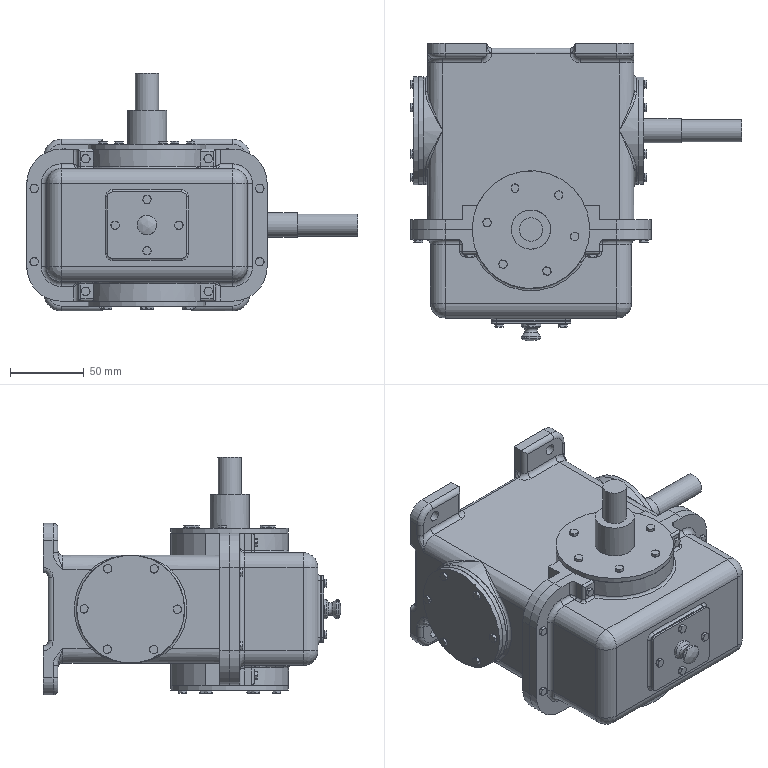Part | STEP file | wolunwogan | 53 solids | 1728 faces | box 225.467 x 202.313 x 161.667 mm | volume 1142690 mm3 | cylinder 603 | plane 488 | cone 320 | spline 232 | torus 76 | sphere 9 | commonest cylinder face diameters 5.933 x216 3.333 x92 101.333 x70 6.667 x60 20 x18 4 x16